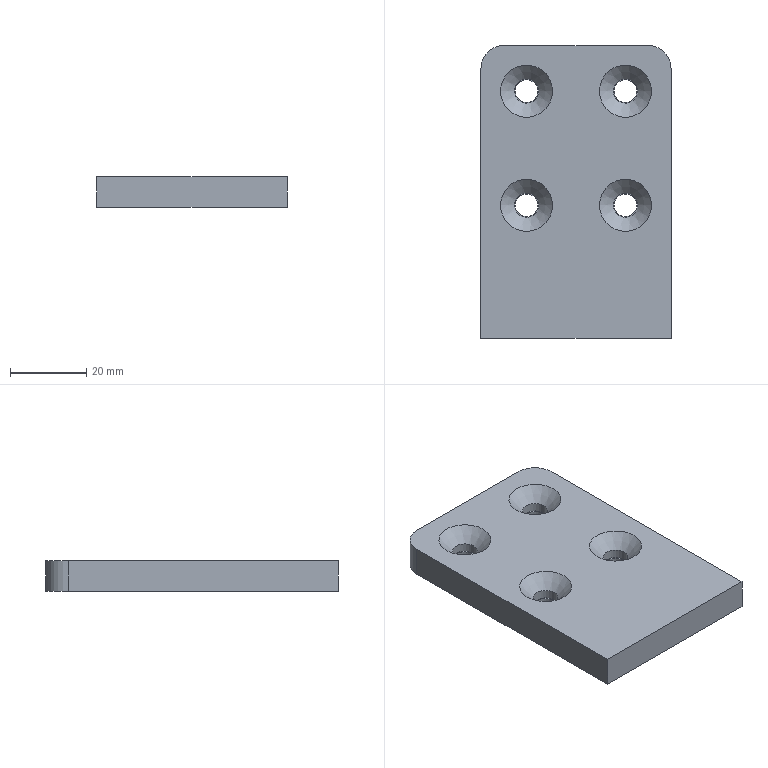Part | STEP file | solid 60 | 1 solid | 24 faces | box 50 x 77 x 8 mm | volume 28929 mm3 | plane 10 | cylinder 10 | cone 4 | commonest cylinder face diameters 6 x4 6.5 x4 12 x2